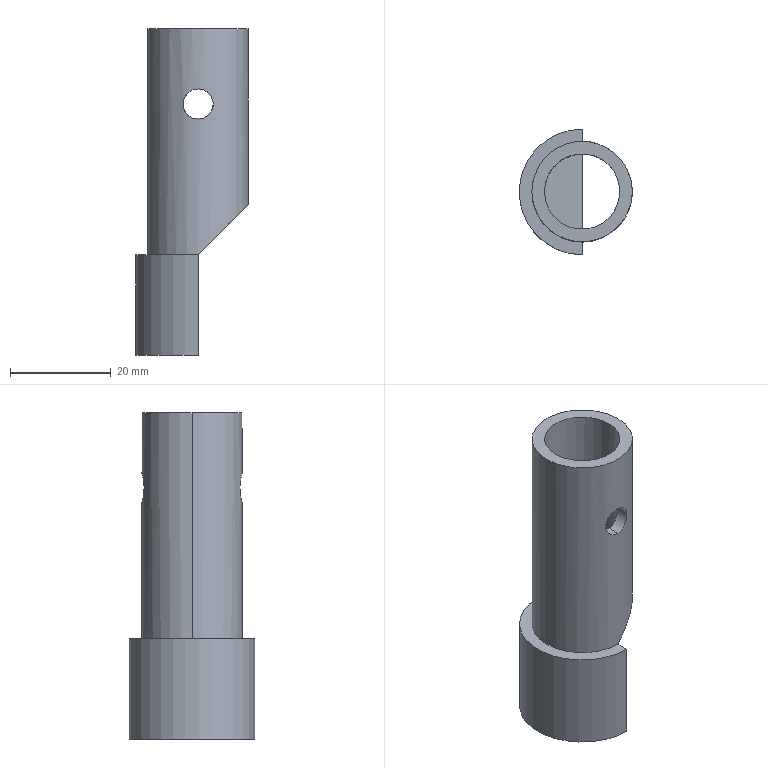Part | SolidWorks | features ICE 3, Extrusion 1, RevCut 1 | 1 solid | 17 faces | box 22.5 x 25 x 65 mm | volume 9681 mm3 | cylinder 9 | plane 6 | sphere 2 | commonest cylinder face diameters 6 x4 15 x2 20 x2 25 x1
STEP:
#1=CARTESIAN_POINT('',(0.,0.,-2.5));
#2=VERTEX_POINT('',#1);
#3=CARTESIAN_POINT('',(0.,0.,-17.5));
#4=VERTEX_POINT('',#3);
#5=CARTESIAN_POINT('',(0.,0.,-10.));
#6=DIRECTION('',(1.,0.,0.));
#7=DIRECTION('',(0.,0.,1.));
#8=AXIS2_PLACEMENT_3D('',#5,#6,#7);
#9=CIRCLE('',#8,7.5);
#10=EDGE_CURVE('',#2,#4,#9,.T.);
#11=ORIENTED_EDGE('',*,*,#10,.T.);
#12=CARTESIAN_POINT('',(0.,0.,-10.));
#13=DIRECTION('',(0.,1.,0.));
#14=DIRECTION('',(0.,0.,1.));
#15=AXIS2_PLACEMENT_3D('',#12,#13,#14);
#16=CIRCLE('',#15,7.5);
#17=EDGE_CURVE('',#4,#2,#16,.T.);
#18=ORIENTED_EDGE('',*,*,#17,.T.);
#19=EDGE_LOOP('',(#11,#18));
#20=FACE_OUTER_BOUND('',#19,.T.);
#21=CARTESIAN_POINT('',(0.,0.,-10.));
#22=DIRECTION('',(0.,-1.,0.));
#23=DIRECTION('',(-1.,0.,0.));
#24=AXIS2_PLACEMENT_3D('',#21,#22,#23);
#25=SPHERICAL_SURFACE('',#24,7.5);
#26=ADVANCED_FACE('',(#20),#25,.F.);
#27=CARTESIAN_POINT('',(0.,-10.,27.));
#28=VERTEX_POINT('',#27);
#29=CARTESIAN_POINT('',(0.,-10.,33.));
#30=VERTEX_POINT('',#29);
#31=CARTESIAN_POINT('',(0.,-10.,27.));
#32=CARTESIAN_POINT('',(-0.1965,-10.,27.));
#33=CARTESIAN_POINT('',(-0.3936,-9.994,27.019));
#34=CARTESIAN_POINT('',(-0.783,-9.971,27.097));
#35=CARTESIAN_POINT('',(-0.9706,-9.954,27.155));
#36=CARTESIAN_POINT('',(-1.332,-9.913,27.305));
#37=CARTESIAN_POINT('',(-1.508,-9.887,27.399));
#38=CARTESIAN_POINT('',(-1.832,-9.832,27.617));
#39=CARTESIAN_POINT('',(-1.983,-9.803,27.74));
#40=CARTESIAN_POINT('',(-2.259,-9.742,28.017));
#41=CARTESIAN_POINT('',(-2.385,-9.712,28.169));
#42=CARTESIAN_POINT('',(-2.601,-9.656,28.493));
#43=CARTESIAN_POINT('',(-2.694,-9.631,28.665));
#44=CARTESIAN_POINT('',(-2.846,-9.587,29.031));
#45=CARTESIAN_POINT('',(-2.903,-9.569,29.218));
#46=CARTESIAN_POINT('',(-2.98,-9.546,29.603));
#47=CARTESIAN_POINT('',(-3.,-9.539,29.802));
#48=CARTESIAN_POINT('',(-3.,-9.539,30.198));
#49=CARTESIAN_POINT('',(-2.981,-9.546,30.393));
#50=CARTESIAN_POINT('',(-2.904,-9.569,30.78));
#51=CARTESIAN_POINT('',(-2.845,-9.587,30.971));
#52=CARTESIAN_POINT('',(-2.62,-9.652,31.513));
#53=CARTESIAN_POINT('',(-2.397,-9.713,31.845));
#54=CARTESIAN_POINT('',(-1.985,-9.802,32.258));
#55=CARTESIAN_POINT('',(-1.832,-9.832,32.384));
#56=CARTESIAN_POINT('',(-1.507,-9.887,32.602));
#57=CARTESIAN_POINT('',(-1.335,-9.912,32.694));
#58=CARTESIAN_POINT('',(-0.973,-9.954,32.845));
#59=CARTESIAN_POINT('',(-0.7815,-9.971,32.903));
#60=CARTESIAN_POINT('',(-0.3956,-9.994,32.98));
#61=CARTESIAN_POINT('',(-0.1994,-10.,33.));
#62=CARTESIAN_POINT('',(0.,-10.,33.));
#63=B_SPLINE_CURVE_WITH_KNOTS('',3,(#31,#32,#33,#34,#35,#36,#37,#38,#39,#40,#41,#42,#43,#44,#45,#46,#47,#48,#49,#50,#51,#52,#53,#54,#55,#56,#57,#58,#59,#60,#61,#62),.UNSPECIFIED.,.F.,.F.,(4,2,2,2,2,2,2,2,2,2,2,2,2,2,2,4),(0.009434,0.01002,0.01061,0.0112,0.01179,0.01238,0.01297,0.01356,0.01415,0.01474,0.01533,0.01651,0.0171,0.01769,0.01828,0.01887),.UNSPECIFIED.);
#64=EDGE_CURVE('',#28,#30,#63,.T.);
#65=ORIENTED_EDGE('',*,*,#64,.F.);
#66=CARTESIAN_POINT('',(0.,-7.5,27.));
#67=VERTEX_POINT('',#66);
#68=CARTESIAN_POINT('',(0.,-10.,27.));
#69=DIRECTION('',(0.,1.,0.));
#70=VECTOR('',#69,1000.);
#71=LINE('',#68,#70);
#72=EDGE_CURVE('',#28,#67,#71,.T.);
#73=ORIENTED_EDGE('',*,*,#72,.T.);
#74=CARTESIAN_POINT('',(0.,-7.5,33.));
#75=VERTEX_POINT('',#74);
#76=CARTESIAN_POINT('',(0.,-7.5,27.));
#77=CARTESIAN_POINT('',(-0.1973,-7.5,27.));
#78=CARTESIAN_POINT('',(-0.3974,-7.492,27.02));
#79=CARTESIAN_POINT('',(-0.7861,-7.461,27.098));
#80=CARTESIAN_POINT('',(-0.9739,-7.439,27.156));
#81=CARTESIAN_POINT('',(-1.337,-7.382,27.307));
#82=CARTESIAN_POINT('',(-1.511,-7.348,27.401));
#83=CARTESIAN_POINT('',(-1.834,-7.274,27.618));
#84=CARTESIAN_POINT('',(-1.985,-7.234,27.742));
#85=CARTESIAN_POINT('',(-2.261,-7.152,28.019));
#86=CARTESIAN_POINT('',(-2.384,-7.112,28.168));
#87=CARTESIAN_POINT('',(-2.6,-7.036,28.49));
#88=CARTESIAN_POINT('',(-2.694,-7.,28.665));
#89=CARTESIAN_POINT('',(-2.845,-6.94,29.027));
#90=CARTESIAN_POINT('',(-2.902,-6.916,29.214));
#91=CARTESIAN_POINT('',(-2.98,-6.883,29.601));
#92=CARTESIAN_POINT('',(-3.,-6.874,29.802));
#93=CARTESIAN_POINT('',(-3.,-6.874,30.197));
#94=CARTESIAN_POINT('',(-2.981,-6.882,30.394));
#95=CARTESIAN_POINT('',(-2.902,-6.916,30.785));
#96=CARTESIAN_POINT('',(-2.844,-6.94,30.974));
#97=CARTESIAN_POINT('',(-2.694,-7.,31.335));
#98=CARTESIAN_POINT('',(-2.6,-7.036,31.509));
#99=CARTESIAN_POINT('',(-2.383,-7.112,31.833));
#100=CARTESIAN_POINT('',(-2.26,-7.153,31.983));
#101=CARTESIAN_POINT('',(-1.985,-7.234,32.258));
#102=CARTESIAN_POINT('',(-1.833,-7.275,32.383));
#103=CARTESIAN_POINT('',(-1.51,-7.348,32.599));
#104=CARTESIAN_POINT('',(-1.339,-7.382,32.692));
#105=CARTESIAN_POINT('',(-0.9736,-7.439,32.845));
#106=CARTESIAN_POINT('',(-0.7847,-7.461,32.902));
#107=CARTESIAN_POINT('',(-0.3992,-7.492,32.98));
#108=CARTESIAN_POINT('',(-0.2004,-7.5,33.));
#109=CARTESIAN_POINT('',(0.,-7.5,33.));
#110=B_SPLINE_CURVE_WITH_KNOTS('',3,(#76,#77,#78,#79,#80,#81,#82,#83,#84,#85,#86,#87,#88,#89,#90,#91,#92,#93,#94,#95,#96,#97,#98,#99,#100,#101,#102,#103,#104,#105,#106,#107,#108,#109),.UNSPECIFIED.,.F.,.F.,(4,2,2,2,2,2,2,2,2,2,2,2,2,2,2,2,4),(0.00948,0.01007,0.01066,0.01126,0.01185,0.01244,0.01303,0.01362,0.01422,0.01481,0.0154,0.01599,0.01658,0.01718,0.01777,0.01836,0.01895),.UNSPECIFIED.);
#111=EDGE_CURVE('',#67,#75,#110,.T.);
#112=ORIENTED_EDGE('',*,*,#111,.T.);
#113=CARTESIAN_POINT('',(0.,-10.,33.));
#114=DIRECTION('',(0.,1.,0.));
#115=VECTOR('',#114,1000.);
#116=LINE('',#113,#115);
#117=EDGE_CURVE('',#30,#75,#116,.T.);
#118=ORIENTED_EDGE('',*,*,#117,.F.);
#119=EDGE_LOOP('',(#65,#73,#112,#118));
#120=FACE_OUTER_BOUND('',#119,.T.);
#121=CARTESIAN_POINT('',(0.,-10.,30.));
#122=DIRECTION('',(0.,1.,0.));
#123=DIRECTION('',(0.,0.,1.));
#124=AXIS2_PLACEMENT_3D('',#121,#122,#123);
#125=CYLINDRICAL_SURFACE('',#124,3.);
#126=ADVANCED_FACE('',(#120),#125,.F.);
#127=CARTESIAN_POINT('',(0.,7.5,33.));
#128=VERTEX_POINT('',#127);
#129=CARTESIAN_POINT('',(0.,7.5,27.));
#130=VERTEX_POINT('',#129);
#131=CARTESIAN_POINT('',(0.,7.5,33.));
#132=CARTESIAN_POINT('',(-0.2005,7.5,33.));
#133=CARTESIAN_POINT('',(-0.3972,7.492,32.98));
#134=CARTESIAN_POINT('',(-0.7836,7.461,32.903));
#135=CARTESIAN_POINT('',(-0.9753,7.439,32.844));
#136=CARTESIAN_POINT('',(-1.338,7.382,32.692));
#137=CARTESIAN_POINT('',(-1.509,7.348,32.6));
#138=CARTESIAN_POINT('',(-1.834,7.274,32.382));
#139=CARTESIAN_POINT('',(-1.986,7.234,32.257));
#140=CARTESIAN_POINT('',(-2.396,7.113,31.846));
#141=CARTESIAN_POINT('',(-2.618,7.03,31.515));
#142=CARTESIAN_POINT('',(-2.844,6.94,30.975));
#143=CARTESIAN_POINT('',(-2.902,6.916,30.784));
#144=CARTESIAN_POINT('',(-2.98,6.883,30.396));
#145=CARTESIAN_POINT('',(-3.,6.874,30.2));
#146=CARTESIAN_POINT('',(-3.,6.874,29.804));
#147=CARTESIAN_POINT('',(-2.98,6.883,29.603));
#148=CARTESIAN_POINT('',(-2.902,6.916,29.216));
#149=CARTESIAN_POINT('',(-2.845,6.94,29.028));
#150=CARTESIAN_POINT('',(-2.692,7.001,28.662));
#151=CARTESIAN_POINT('',(-2.6,7.036,28.491));
#152=CARTESIAN_POINT('',(-2.383,7.112,28.168));
#153=CARTESIAN_POINT('',(-2.258,7.153,28.015));
#154=CARTESIAN_POINT('',(-1.983,7.234,27.741));
#155=CARTESIAN_POINT('',(-1.834,7.274,27.618));
#156=CARTESIAN_POINT('',(-1.51,7.348,27.4));
#157=CARTESIAN_POINT('',(-1.335,7.383,27.306));
#158=CARTESIAN_POINT('',(-0.974,7.439,27.156));
#159=CARTESIAN_POINT('',(-0.7864,7.461,27.098));
#160=CARTESIAN_POINT('',(-0.3955,7.492,27.02));
#161=CARTESIAN_POINT('',(-0.1975,7.5,27.));
#162=CARTESIAN_POINT('',(0.,7.5,27.));
#163=B_SPLINE_CURVE_WITH_KNOTS('',3,(#131,#132,#133,#134,#135,#136,#137,#138,#139,#140,#141,#142,#143,#144,#145,#146,#147,#148,#149,#150,#151,#152,#153,#154,#155,#156,#157,#158,#159,#160,#161,#162),.UNSPECIFIED.,.F.,.F.,(4,2,2,2,2,2,2,2,2,2,2,2,2,2,2,4),(0.,0.0005925,0.001185,0.001777,0.00237,0.003555,0.004147,0.00474,0.005332,0.005925,0.006517,0.00711,0.007702,0.008295,0.008887,0.00948),.UNSPECIFIED.);
#164=EDGE_CURVE('',#128,#130,#163,.T.);
#165=ORIENTED_EDGE('',*,*,#164,.T.);
#166=CARTESIAN_POINT('',(0.,10.,27.));
#167=VERTEX_POINT('',#166);
#168=CARTESIAN_POINT('',(0.,-10.,27.));
#169=DIRECTION('',(0.,1.,0.));
#170=VECTOR('',#169,1000.);
#171=LINE('',#168,#170);
#172=EDGE_CURVE('',#130,#167,#171,.T.);
#173=ORIENTED_EDGE('',*,*,#172,.T.);
#174=CARTESIAN_POINT('',(0.,10.,33.));
#175=VERTEX_POINT('',#174);
#176=CARTESIAN_POINT('',(0.,10.,33.));
#177=CARTESIAN_POINT('',(-0.1995,10.,33.));
#178=CARTESIAN_POINT('',(-0.3954,9.994,32.98));
#179=CARTESIAN_POINT('',(-0.7804,9.971,32.903));
#180=CARTESIAN_POINT('',(-0.9716,9.954,32.845));
#181=CARTESIAN_POINT('',(-1.334,9.912,32.694));
#182=CARTESIAN_POINT('',(-1.506,9.887,32.602));
#183=CARTESIAN_POINT('',(-1.832,9.832,32.384));
#184=CARTESIAN_POINT('',(-1.985,9.802,32.258));
#185=CARTESIAN_POINT('',(-2.397,9.713,31.845));
#186=CARTESIAN_POINT('',(-2.62,9.652,31.513));
#187=CARTESIAN_POINT('',(-2.845,9.587,30.972));
#188=CARTESIAN_POINT('',(-2.903,9.569,30.782));
#189=CARTESIAN_POINT('',(-2.981,9.546,30.394));
#190=CARTESIAN_POINT('',(-3.,9.539,30.198));
#191=CARTESIAN_POINT('',(-3.,9.539,29.804));
#192=CARTESIAN_POINT('',(-2.98,9.546,29.604));
#193=CARTESIAN_POINT('',(-2.903,9.569,29.219));
#194=CARTESIAN_POINT('',(-2.846,9.587,29.031));
#195=CARTESIAN_POINT('',(-2.694,9.63,28.666));
#196=CARTESIAN_POINT('',(-2.601,9.656,28.493));
#197=CARTESIAN_POINT('',(-2.384,9.712,28.169));
#198=CARTESIAN_POINT('',(-2.259,9.743,28.016));
#199=CARTESIAN_POINT('',(-1.982,9.803,27.74));
#200=CARTESIAN_POINT('',(-1.832,9.832,27.616));
#201=CARTESIAN_POINT('',(-1.508,9.887,27.399));
#202=CARTESIAN_POINT('',(-1.332,9.913,27.305));
#203=CARTESIAN_POINT('',(-0.9703,9.954,27.154));
#204=CARTESIAN_POINT('',(-0.7831,9.971,27.097));
#205=CARTESIAN_POINT('',(-0.3956,9.994,27.02));
#206=CARTESIAN_POINT('',(-0.1965,10.,27.));
#207=CARTESIAN_POINT('',(0.,10.,27.));
#208=B_SPLINE_CURVE_WITH_KNOTS('',3,(#176,#177,#178,#179,#180,#181,#182,#183,#184,#185,#186,#187,#188,#189,#190,#191,#192,#193,#194,#195,#196,#197,#198,#199,#200,#201,#202,#203,#204,#205,#206,#207),.UNSPECIFIED.,.F.,.F.,(4,2,2,2,2,2,2,2,2,2,2,2,2,2,2,4),(0.,0.0005896,0.001179,0.001769,0.002359,0.003538,0.004127,0.004717,0.005307,0.005896,0.006486,0.007076,0.007665,0.008255,0.008844,0.009434),.UNSPECIFIED.);
#209=EDGE_CURVE('',#175,#167,#208,.T.);
#210=ORIENTED_EDGE('',*,*,#209,.F.);
#211=CARTESIAN_POINT('',(0.,-10.,33.));
#212=DIRECTION('',(0.,1.,0.));
#213=VECTOR('',#212,1000.);
#214=LINE('',#211,#213);
#215=EDGE_CURVE('',#128,#175,#214,.T.);
#216=ORIENTED_EDGE('',*,*,#215,.F.);
#217=EDGE_LOOP('',(#165,#173,#210,#216));
#218=FACE_OUTER_BOUND('',#217,.T.);
#219=CARTESIAN_POINT('',(0.,-10.,30.));
#220=DIRECTION('',(0.,1.,0.));
#221=DIRECTION('',(0.,0.,1.));
#222=AXIS2_PLACEMENT_3D('',#219,#220,#221);
#223=CYLINDRICAL_SURFACE('',#222,3.);
#224=ADVANCED_FACE('',(#218),#223,.F.);
#225=CARTESIAN_POINT('',(0.,-7.5,33.));
#226=CARTESIAN_POINT('',(0.2005,-7.5,33.));
#227=CARTESIAN_POINT('',(0.3972,-7.492,32.98));
#228=CARTESIAN_POINT('',(0.7836,-7.461,32.903));
#229=CARTESIAN_POINT('',(0.9753,-7.439,32.844));
#230=CARTESIAN_POINT('',(1.338,-7.382,32.692));
#231=CARTESIAN_POINT('',(1.509,-7.348,32.6));
#232=CARTESIAN_POINT('',(1.834,-7.274,32.382));
#233=CARTESIAN_POINT('',(1.986,-7.234,32.257));
#234=CARTESIAN_POINT('',(2.396,-7.113,31.846));
#235=CARTESIAN_POINT('',(2.618,-7.03,31.515));
#236=CARTESIAN_POINT('',(2.844,-6.94,30.975));
#237=CARTESIAN_POINT('',(2.902,-6.916,30.784));
#238=CARTESIAN_POINT('',(2.98,-6.883,30.396));
#239=CARTESIAN_POINT('',(3.,-6.874,30.2));
#240=CARTESIAN_POINT('',(3.,-6.874,29.804));
#241=CARTESIAN_POINT('',(2.98,-6.883,29.603));
#242=CARTESIAN_POINT('',(2.902,-6.916,29.216));
#243=CARTESIAN_POINT('',(2.845,-6.94,29.028));
#244=CARTESIAN_POINT('',(2.692,-7.001,28.662));
#245=CARTESIAN_POINT('',(2.6,-7.036,28.491));
#246=CARTESIAN_POINT('',(2.383,-7.112,28.168));
#247=CARTESIAN_POINT('',(2.258,-7.153,28.015));
#248=CARTESIAN_POINT('',(1.983,-7.234,27.741));
#249=CARTESIAN_POINT('',(1.834,-7.274,27.618));
#250=CARTESIAN_POINT('',(1.51,-7.348,27.4));
#251=CARTESIAN_POINT('',(1.335,-7.383,27.306));
#252=CARTESIAN_POINT('',(0.974,-7.439,27.156));
#253=CARTESIAN_POINT('',(0.7864,-7.461,27.098));
#254=CARTESIAN_POINT('',(0.3955,-7.492,27.02));
#255=CARTESIAN_POINT('',(0.1975,-7.5,27.));
#256=CARTESIAN_POINT('',(0.,-7.5,27.));
#257=B_SPLINE_CURVE_WITH_KNOTS('',3,(#225,#226,#227,#228,#229,#230,#231,#232,#233,#234,#235,#236,#237,#238,#239,#240,#241,#242,#243,#244,#245,#246,#247,#248,#249,#250,#251,#252,#253,#254,#255,#256),.UNSPECIFIED.,.F.,.F.,(4,2,2,2,2,2,2,2,2,2,2,2,2,2,2,4),(0.,0.0005925,0.001185,0.001777,0.00237,0.003555,0.004147,0.00474,0.005332,0.005925,0.006517,0.00711,0.007702,0.008295,0.008887,0.00948),.UNSPECIFIED.);
#258=EDGE_CURVE('',#75,#67,#257,.T.);
#259=ORIENTED_EDGE('',*,*,#258,.F.);
#260=ORIENTED_EDGE('',*,*,#111,.F.);
#261=EDGE_LOOP('',(#259,#260));
#262=FACE_BOUND('',#261,.T.);
#263=CARTESIAN_POINT('',(-7.5,0.,45.));
#264=VERTEX_POINT('',#263);
#265=CARTESIAN_POINT('',(7.5,0.,45.));
#266=VERTEX_POINT('',#265);
#267=CARTESIAN_POINT('',(0.,0.,45.));
#268=DIRECTION('',(0.,0.,1.));
#269=DIRECTION('',(1.,0.,0.));
#270=AXIS2_PLACEMENT_3D('',#267,#268,#269);
#271=CIRCLE('',#270,7.5);
#272=EDGE_CURVE('',#264,#266,#271,.T.);
#273=ORIENTED_EDGE('',*,*,#272,.T.);
#274=CARTESIAN_POINT('',(7.5,0.,7.5));
#275=VERTEX_POINT('',#274);
#276=CARTESIAN_POINT('',(7.5,0.,45.));
#277=DIRECTION('',(0.,0.,-1.));
#278=VECTOR('',#277,1000.);
#279=LINE('',#276,#278);
#280=EDGE_CURVE('',#266,#275,#279,.T.);
#281=ORIENTED_EDGE('',*,*,#280,.T.);
#282=CARTESIAN_POINT('',(0.,-7.5,0.));
#283=VERTEX_POINT('',#282);
#284=CARTESIAN_POINT('',(0.,-7.5,0.));
#285=CARTESIAN_POINT('',(4.393,-7.5,4.393));
#286=CARTESIAN_POINT('',(7.5,-4.393,7.5));
#287=CARTESIAN_POINT('',(7.5,0.,7.5));
#288=(BOUNDED_CURVE()B_SPLINE_CURVE(3,(#284,#285,#286,#287),.UNSPECIFIED.,.F.,.F.)B_SPLINE_CURVE_WITH_KNOTS((4,4),(1.571,3.142),.UNSPECIFIED.)CURVE()GEOMETRIC_REPRESENTATION_ITEM()RATIONAL_B_SPLINE_CURVE((1.,0.8047,0.8047,1.))REPRESENTATION_ITEM(''));
#289=EDGE_CURVE('',#283,#275,#288,.T.);
#290=ORIENTED_EDGE('',*,*,#289,.F.);
#291=CARTESIAN_POINT('',(-7.5,0.,0.));
#292=VERTEX_POINT('',#291);
#293=CARTESIAN_POINT('',(0.,0.,0.));
#294=DIRECTION('',(0.,0.,1.));
#295=DIRECTION('',(1.,0.,0.));
#296=AXIS2_PLACEMENT_3D('',#293,#294,#295);
#297=CIRCLE('',#296,7.5);
#298=EDGE_CURVE('',#292,#283,#297,.T.);
#299=ORIENTED_EDGE('',*,*,#298,.F.);
#300=CARTESIAN_POINT('',(-7.5,0.,45.));
#301=DIRECTION('',(0.,0.,-1.));
#302=VECTOR('',#301,1000.);
#303=LINE('',#300,#302);
#304=EDGE_CURVE('',#264,#292,#303,.T.);
#305=ORIENTED_EDGE('',*,*,#304,.F.);
#306=EDGE_LOOP('',(#273,#281,#290,#299,#305));
#307=FACE_OUTER_BOUND('',#306,.T.);
#308=CARTESIAN_POINT('',(0.,0.,45.));
#309=DIRECTION('',(0.,0.,-1.));
#310=DIRECTION('',(-1.,0.,0.));
#311=AXIS2_PLACEMENT_3D('',#308,#309,#310);
#312=CYLINDRICAL_SURFACE('',#311,7.5);
#313=ADVANCED_FACE('',(#262,#307),#312,.F.);
#314=ORIENTED_EDGE('',*,*,#209,.T.);
#315=CARTESIAN_POINT('',(0.,10.,27.));
#316=CARTESIAN_POINT('',(0.1965,10.,27.));
#317=CARTESIAN_POINT('',(0.3936,9.994,27.019));
#318=CARTESIAN_POINT('',(0.783,9.971,27.097));
#319=CARTESIAN_POINT('',(0.9706,9.954,27.155));
#320=CARTESIAN_POINT('',(1.332,9.913,27.305));
#321=CARTESIAN_POINT('',(1.508,9.887,27.399));
#322=CARTESIAN_POINT('',(1.832,9.832,27.617));
#323=CARTESIAN_POINT('',(1.983,9.803,27.74));
#324=CARTESIAN_POINT('',(2.259,9.742,28.017));
#325=CARTESIAN_POINT('',(2.385,9.712,28.169));
#326=CARTESIAN_POINT('',(2.601,9.656,28.493));
#327=CARTESIAN_POINT('',(2.694,9.631,28.665));
#328=CARTESIAN_POINT('',(2.846,9.587,29.031));
#329=CARTESIAN_POINT('',(2.903,9.569,29.218));
#330=CARTESIAN_POINT('',(2.98,9.546,29.603));
#331=CARTESIAN_POINT('',(3.,9.539,29.802));
#332=CARTESIAN_POINT('',(3.,9.539,30.198));
#333=CARTESIAN_POINT('',(2.981,9.546,30.393));
#334=CARTESIAN_POINT('',(2.904,9.569,30.78));
#335=CARTESIAN_POINT('',(2.845,9.587,30.971));
#336=CARTESIAN_POINT('',(2.62,9.652,31.513));
#337=CARTESIAN_POINT('',(2.397,9.713,31.845));
#338=CARTESIAN_POINT('',(1.985,9.802,32.258));
#339=CARTESIAN_POINT('',(1.832,9.832,32.384));
#340=CARTESIAN_POINT('',(1.507,9.887,32.602));
#341=CARTESIAN_POINT('',(1.335,9.912,32.694));
#342=CARTESIAN_POINT('',(0.973,9.954,32.845));
#343=CARTESIAN_POINT('',(0.7815,9.971,32.903));
#344=CARTESIAN_POINT('',(0.3956,9.994,32.98));
#345=CARTESIAN_POINT('',(0.1994,10.,33.));
#346=CARTESIAN_POINT('',(0.,10.,33.));
#347=B_SPLINE_CURVE_WITH_KNOTS('',3,(#315,#316,#317,#318,#319,#320,#321,#322,#323,#324,#325,#326,#327,#328,#329,#330,#331,#332,#333,#334,#335,#336,#337,#338,#339,#340,#341,#342,#343,#344,#345,#346),.UNSPECIFIED.,.F.,.F.,(4,2,2,2,2,2,2,2,2,2,2,2,2,2,2,4),(0.009434,0.01002,0.01061,0.0112,0.01179,0.01238,0.01297,0.01356,0.01415,0.01474,0.01533,0.01651,0.0171,0.01769,0.01828,0.01887),.UNSPECIFIED.);
#348=EDGE_CURVE('',#167,#175,#347,.T.);
#349=ORIENTED_EDGE('',*,*,#348,.T.);
#350=EDGE_LOOP('',(#314,#349));
#351=FACE_BOUND('',#350,.T.);
#352=CARTESIAN_POINT('',(10.,0.,45.));
#353=VERTEX_POINT('',#352);
#354=CARTESIAN_POINT('',(-10.,0.,45.));
#355=VERTEX_POINT('',#354);
#356=CARTESIAN_POINT('',(0.,0.,45.));
#357=DIRECTION('',(0.,0.,1.));
#358=DIRECTION('',(1.,0.,0.));
#359=AXIS2_PLACEMENT_3D('',#356,#357,#358);
#360=CIRCLE('',#359,10.);
#361=EDGE_CURVE('',#353,#355,#360,.T.);
#362=ORIENTED_EDGE('',*,*,#361,.F.);
#363=CARTESIAN_POINT('',(10.,0.,10.));
#364=VERTEX_POINT('',#363);
#365=CARTESIAN_POINT('',(10.,0.,45.));
#366=DIRECTION('',(0.,0.,-1.));
#367=VECTOR('',#366,1000.);
#368=LINE('',#365,#367);
#369=EDGE_CURVE('',#353,#364,#368,.T.);
#370=ORIENTED_EDGE('',*,*,#369,.T.);
#371=CARTESIAN_POINT('',(0.,10.,0.));
#372=VERTEX_POINT('',#371);
#373=CARTESIAN_POINT('',(10.,0.,10.));
#374=CARTESIAN_POINT('',(10.,5.858,10.));
#375=CARTESIAN_POINT('',(5.858,10.,5.858));
#376=CARTESIAN_POINT('',(0.,10.,0.));
#377=(BOUNDED_CURVE()B_SPLINE_CURVE(3,(#373,#374,#375,#376),.UNSPECIFIED.,.F.,.F.)B_SPLINE_CURVE_WITH_KNOTS((4,4),(3.142,4.712),.UNSPECIFIED.)CURVE()GEOMETRIC_REPRESENTATION_ITEM()RATIONAL_B_SPLINE_CURVE((1.,0.8047,0.8047,1.))REPRESENTATION_ITEM(''));
#378=EDGE_CURVE('',#364,#372,#377,.T.);
#379=ORIENTED_EDGE('',*,*,#378,.T.);
#380=CARTESIAN_POINT('',(-10.,0.,0.));
#381=VERTEX_POINT('',#380);
#382=CARTESIAN_POINT('',(0.,0.,0.));
#383=DIRECTION('',(0.,0.,-1.));
#384=DIRECTION('',(-1.,0.,0.));
#385=AXIS2_PLACEMENT_3D('',#382,#383,#384);
#386=CIRCLE('',#385,10.);
#387=EDGE_CURVE('',#381,#372,#386,.T.);
#388=ORIENTED_EDGE('',*,*,#387,.F.);
#389=CARTESIAN_POINT('',(-10.,0.,45.));
#390=DIRECTION('',(0.,0.,-1.));
#391=VECTOR('',#390,1000.);
#392=LINE('',#389,#391);
#393=EDGE_CURVE('',#355,#381,#392,.T.);
#394=ORIENTED_EDGE('',*,*,#393,.F.);
#395=EDGE_LOOP('',(#362,#370,#379,#388,#394));
#396=FACE_OUTER_BOUND('',#395,.T.);
#397=CARTESIAN_POINT('',(0.,0.,45.));
#398=DIRECTION('',(0.,0.,-1.));
#399=DIRECTION('',(-1.,0.,0.));
#400=AXIS2_PLACEMENT_3D('',#397,#398,#399);
#401=CYLINDRICAL_SURFACE('',#400,10.);
#402=ADVANCED_FACE('',(#351,#396),#401,.T.);
#403=CARTESIAN_POINT('',(0.,0.,45.));
#404=DIRECTION('',(0.,0.,1.));
#405=DIRECTION('',(1.,0.,0.));
#406=AXIS2_PLACEMENT_3D('',#403,#404,#405);
#407=CIRCLE('',#406,10.);
#408=EDGE_CURVE('',#355,#353,#407,.T.);
#409=ORIENTED_EDGE('',*,*,#408,.T.);
#410=ORIENTED_EDGE('',*,*,#361,.T.);
#411=EDGE_LOOP('',(#409,#410));
#412=FACE_OUTER_BOUND('',#411,.T.);
#413=ORIENTED_EDGE('',*,*,#272,.F.);
#414=CARTESIAN_POINT('',(0.,0.,45.));
#415=DIRECTION('',(0.,0.,1.));
#416=DIRECTION('',(1.,0.,0.));
#417=AXIS2_PLACEMENT_3D('',#414,#415,#416);
#418=CIRCLE('',#417,7.5);
#419=EDGE_CURVE('',#266,#264,#418,.T.);
#420=ORIENTED_EDGE('',*,*,#419,.F.);
#421=EDGE_LOOP('',(#413,#420));
#422=FACE_BOUND('',#421,.T.);
#423=CARTESIAN_POINT('',(0.,0.,45.));
#424=DIRECTION('',(0.,0.,1.));
#425=DIRECTION('',(1.,0.,0.));
#426=AXIS2_PLACEMENT_3D('',#423,#424,#425);
#427=PLANE('',#426);
#428=ADVANCED_FACE('',(#412,#422),#427,.T.);
#429=ORIENTED_EDGE('',*,*,#369,.F.);
#430=ORIENTED_EDGE('',*,*,#408,.F.);
#431=ORIENTED_EDGE('',*,*,#393,.T.);
#432=CARTESIAN_POINT('',(0.,-10.,0.));
#433=VERTEX_POINT('',#432);
#434=CARTESIAN_POINT('',(0.,0.,0.));
#435=DIRECTION('',(0.,0.,-1.));
#436=DIRECTION('',(-1.,0.,0.));
#437=AXIS2_PLACEMENT_3D('',#434,#435,#436);
#438=CIRCLE('',#437,10.);
#439=EDGE_CURVE('',#433,#381,#438,.T.);
#440=ORIENTED_EDGE('',*,*,#439,.F.);
#441=CARTESIAN_POINT('',(0.,-10.,0.));
#442=CARTESIAN_POINT('',(5.858,-10.,5.858));
#443=CARTESIAN_POINT('',(10.,-5.858,10.));
#444=CARTESIAN_POINT('',(10.,0.,10.));
#445=(BOUNDED_CURVE()B_SPLINE_CURVE(3,(#441,#442,#443,#444),.UNSPECIFIED.,.F.,.F.)B_SPLINE_CURVE_WITH_KNOTS((4,4),(1.571,3.142),.UNSPECIFIED.)CURVE()GEOMETRIC_REPRESENTATION_ITEM()RATIONAL_B_SPLINE_CURVE((1.,0.8047,0.8047,1.))REPRESENTATION_ITEM(''));
#446=EDGE_CURVE('',#433,#364,#445,.T.);
#447=ORIENTED_EDGE('',*,*,#446,.T.);
#448=EDGE_LOOP('',(#429,#430,#431,#440,#447));
#449=FACE_OUTER_BOUND('',#448,.T.);
#450=CARTESIAN_POINT('',(0.,-10.,33.));
#451=CARTESIAN_POINT('',(0.1995,-10.,33.));
#452=CARTESIAN_POINT('',(0.3954,-9.994,32.98));
#453=CARTESIAN_POINT('',(0.7804,-9.971,32.903));
#454=CARTESIAN_POINT('',(0.9716,-9.954,32.845));
#455=CARTESIAN_POINT('',(1.334,-9.912,32.694));
#456=CARTESIAN_POINT('',(1.506,-9.887,32.602));
#457=CARTESIAN_POINT('',(1.832,-9.832,32.384));
#458=CARTESIAN_POINT('',(1.985,-9.802,32.258));
#459=CARTESIAN_POINT('',(2.397,-9.713,31.845));
#460=CARTESIAN_POINT('',(2.62,-9.652,31.513));
#461=CARTESIAN_POINT('',(2.845,-9.587,30.972));
#462=CARTESIAN_POINT('',(2.903,-9.569,30.782));
#463=CARTESIAN_POINT('',(2.981,-9.546,30.394));
#464=CARTESIAN_POINT('',(3.,-9.539,30.198));
#465=CARTESIAN_POINT('',(3.,-9.539,29.804));
#466=CARTESIAN_POINT('',(2.98,-9.546,29.604));
#467=CARTESIAN_POINT('',(2.903,-9.569,29.219));
#468=CARTESIAN_POINT('',(2.846,-9.587,29.031));
#469=CARTESIAN_POINT('',(2.694,-9.63,28.666));
#470=CARTESIAN_POINT('',(2.601,-9.656,28.493));
#471=CARTESIAN_POINT('',(2.384,-9.712,28.169));
#472=CARTESIAN_POINT('',(2.259,-9.743,28.016));
#473=CARTESIAN_POINT('',(1.982,-9.803,27.74));
#474=CARTESIAN_POINT('',(1.832,-9.832,27.616));
#475=CARTESIAN_POINT('',(1.508,-9.887,27.399));
#476=CARTESIAN_POINT('',(1.332,-9.913,27.305));
#477=CARTESIAN_POINT('',(0.9703,-9.954,27.154));
#478=CARTESIAN_POINT('',(0.7831,-9.971,27.097));
#479=CARTESIAN_POINT('',(0.3956,-9.994,27.02));
#480=CARTESIAN_POINT('',(0.1965,-10.,27.));
#481=CARTESIAN_POINT('',(0.,-10.,27.));
#482=B_SPLINE_CURVE_WITH_KNOTS('',3,(#450,#451,#452,#453,#454,#455,#456,#457,#458,#459,#460,#461,#462,#463,#464,#465,#466,#467,#468,#469,#470,#471,#472,#473,#474,#475,#476,#477,#478,#479,#480,#481),.UNSPECIFIED.,.F.,.F.,(4,2,2,2,2,2,2,2,2,2,2,2,2,2,2,4),(0.,0.0005896,0.001179,0.001769,0.002359,0.003538,0.004127,0.004717,0.005307,0.005896,0.006486,0.007076,0.007665,0.008255,0.008844,0.009434),.UNSPECIFIED.);
#483=EDGE_CURVE('',#30,#28,#482,.T.);
#484=ORIENTED_EDGE('',*,*,#483,.T.);
#485=ORIENTED_EDGE('',*,*,#64,.T.);
#486=EDGE_LOOP('',(#484,#485));
#487=FACE_BOUND('',#486,.T.);
#488=CARTESIAN_POINT('',(0.,0.,45.));
#489=DIRECTION('',(0.,0.,-1.));
#490=DIRECTION('',(-1.,0.,0.));
#491=AXIS2_PLACEMENT_3D('',#488,#489,#490);
#492=CYLINDRICAL_SURFACE('',#491,10.);
#493=ADVANCED_FACE('',(#449,#487),#492,.T.);
#494=ORIENTED_EDGE('',*,*,#280,.F.);
#495=ORIENTED_EDGE('',*,*,#419,.T.);
#496=ORIENTED_EDGE('',*,*,#304,.T.);
#497=CARTESIAN_POINT('',(0.,7.5,0.));
#498=VERTEX_POINT('',#497);
#499=CARTESIAN_POINT('',(0.,0.,0.));
#500=DIRECTION('',(0.,0.,1.));
#501=DIRECTION('',(1.,0.,0.));
#502=AXIS2_PLACEMENT_3D('',#499,#500,#501);
#503=CIRCLE('',#502,7.5);
#504=EDGE_CURVE('',#498,#292,#503,.T.);
#505=ORIENTED_EDGE('',*,*,#504,.F.);
#506=CARTESIAN_POINT('',(7.5,0.,7.5));
#507=CARTESIAN_POINT('',(7.5,4.393,7.5));
#508=CARTESIAN_POINT('',(4.393,7.5,4.393));
#509=CARTESIAN_POINT('',(0.,7.5,0.));
#510=(BOUNDED_CURVE()B_SPLINE_CURVE(3,(#506,#507,#508,#509),.UNSPECIFIED.,.F.,.F.)B_SPLINE_CURVE_WITH_KNOTS((4,4),(3.142,4.712),.UNSPECIFIED.)CURVE()GEOMETRIC_REPRESENTATION_ITEM()RATIONAL_B_SPLINE_CURVE((1.,0.8047,0.8047,1.))REPRESENTATION_ITEM(''));
#511=EDGE_CURVE('',#275,#498,#510,.T.);
#512=ORIENTED_EDGE('',*,*,#511,.F.);
#513=EDGE_LOOP('',(#494,#495,#496,#505,#512));
#514=FACE_OUTER_BOUND('',#513,.T.);
#515=ORIENTED_EDGE('',*,*,#164,.F.);
#516=CARTESIAN_POINT('',(0.,7.5,27.));
#517=CARTESIAN_POINT('',(0.1973,7.5,27.));
#518=CARTESIAN_POINT('',(0.3974,7.492,27.02));
#519=CARTESIAN_POINT('',(0.7861,7.461,27.098));
#520=CARTESIAN_POINT('',(0.9739,7.439,27.156));
#521=CARTESIAN_POINT('',(1.337,7.382,27.307));
#522=CARTESIAN_POINT('',(1.511,7.348,27.401));
#523=CARTESIAN_POINT('',(1.834,7.274,27.618));
#524=CARTESIAN_POINT('',(1.985,7.234,27.742));
#525=CARTESIAN_POINT('',(2.261,7.152,28.019));
#526=CARTESIAN_POINT('',(2.384,7.112,28.168));
#527=CARTESIAN_POINT('',(2.6,7.036,28.49));
#528=CARTESIAN_POINT('',(2.694,7.,28.665));
#529=CARTESIAN_POINT('',(2.845,6.94,29.027));
#530=CARTESIAN_POINT('',(2.902,6.916,29.214));
#531=CARTESIAN_POINT('',(2.98,6.883,29.601));
#532=CARTESIAN_POINT('',(3.,6.874,29.802));
#533=CARTESIAN_POINT('',(3.,6.874,30.197));
#534=CARTESIAN_POINT('',(2.981,6.882,30.394));
#535=CARTESIAN_POINT('',(2.902,6.916,30.785));
#536=CARTESIAN_POINT('',(2.844,6.94,30.974));
#537=CARTESIAN_POINT('',(2.694,7.,31.335));
#538=CARTESIAN_POINT('',(2.6,7.036,31.509));
#539=CARTESIAN_POINT('',(2.383,7.112,31.833));
#540=CARTESIAN_POINT('',(2.26,7.153,31.983));
#541=CARTESIAN_POINT('',(1.985,7.234,32.258));
#542=CARTESIAN_POINT('',(1.833,7.275,32.383));
#543=CARTESIAN_POINT('',(1.51,7.348,32.599));
#544=CARTESIAN_POINT('',(1.339,7.382,32.692));
#545=CARTESIAN_POINT('',(0.9736,7.439,32.845));
#546=CARTESIAN_POINT('',(0.7847,7.461,32.902));
#547=CARTESIAN_POINT('',(0.3992,7.492,32.98));
#548=CARTESIAN_POINT('',(0.2004,7.5,33.));
#549=CARTESIAN_POINT('',(0.,7.5,33.));
#550=B_SPLINE_CURVE_WITH_KNOTS('',3,(#516,#517,#518,#519,#520,#521,#522,#523,#524,#525,#526,#527,#528,#529,#530,#531,#532,#533,#534,#535,#536,#537,#538,#539,#540,#541,#542,#543,#544,#545,#546,#547,#548,#549),.UNSPECIFIED.,.F.,.F.,(4,2,2,2,2,2,2,2,2,2,2,2,2,2,2,2,4),(0.00948,0.01007,0.01066,0.01126,0.01185,0.01244,0.01303,0.01362,0.01422,0.01481,0.0154,0.01599,0.01658,0.01718,0.01777,0.01836,0.01895),.UNSPECIFIED.);
#551=EDGE_CURVE('',#130,#128,#550,.T.);
#552=ORIENTED_EDGE('',*,*,#551,.F.);
#553=EDGE_LOOP('',(#515,#552));
#554=FACE_BOUND('',#553,.T.);
#555=CARTESIAN_POINT('',(0.,0.,45.));
#556=DIRECTION('',(0.,0.,-1.));
#557=DIRECTION('',(-1.,0.,0.));
#558=AXIS2_PLACEMENT_3D('',#555,#556,#557);
#559=CYLINDRICAL_SURFACE('',#558,7.5);
#560=ADVANCED_FACE('',(#514,#554),#559,.F.);
#561=ORIENTED_EDGE('',*,*,#172,.F.);
#562=ORIENTED_EDGE('',*,*,#551,.T.);
#563=ORIENTED_EDGE('',*,*,#215,.T.);
#564=ORIENTED_EDGE('',*,*,#348,.F.);
#565=EDGE_LOOP('',(#561,#562,#563,#564));
#566=FACE_OUTER_BOUND('',#565,.T.);
#567=CARTESIAN_POINT('',(0.,-10.,30.));
#568=DIRECTION('',(0.,1.,0.));
#569=DIRECTION('',(0.,0.,1.));
#570=AXIS2_PLACEMENT_3D('',#567,#568,#569);
#571=CYLINDRICAL_SURFACE('',#570,3.);
#572=ADVANCED_FACE('',(#566),#571,.F.);
#573=ORIENTED_EDGE('',*,*,#72,.F.);
#574=ORIENTED_EDGE('',*,*,#483,.F.);
#575=ORIENTED_EDGE('',*,*,#117,.T.);
#576=ORIENTED_EDGE('',*,*,#258,.T.);
#577=EDGE_LOOP('',(#573,#574,#575,#576));
#578=FACE_OUTER_BOUND('',#577,.T.);
#579=CARTESIAN_POINT('',(0.,-10.,30.));
#580=DIRECTION('',(0.,1.,0.));
#581=DIRECTION('',(0.,0.,1.));
#582=AXIS2_PLACEMENT_3D('',#579,#580,#581);
#583=CYLINDRICAL_SURFACE('',#582,3.);
#584=ADVANCED_FACE('',(#578),#583,.F.);
#585=ORIENTED_EDGE('',*,*,#504,.T.);
#586=ORIENTED_EDGE('',*,*,#298,.T.);
#587=CARTESIAN_POINT('',(0.,-12.5,0.));
#588=DIRECTION('',(0.,1.,0.));
#589=VECTOR('',#588,1000.);
#590=LINE('',#587,#589);
#591=EDGE_CURVE('',#283,#498,#590,.T.);
#592=ORIENTED_EDGE('',*,*,#591,.T.);
#593=EDGE_LOOP('',(#585,#586,#592));
#594=FACE_OUTER_BOUND('',#593,.T.);
#595=CARTESIAN_POINT('',(0.,0.,0.));
#596=DIRECTION('',(0.,0.,-1.));
#597=DIRECTION('',(-1.,0.,0.));
#598=AXIS2_PLACEMENT_3D('',#595,#596,#597);
#599=PLANE('',#598);
#600=ADVANCED_FACE('',(#594),#599,.F.);
#601=CARTESIAN_POINT('',(0.,-12.5,-20.));
#602=VERTEX_POINT('',#601);
#603=CARTESIAN_POINT('',(0.,12.5,-20.));
#604=VERTEX_POINT('',#603);
#605=CARTESIAN_POINT('',(0.,0.,-20.));
#606=DIRECTION('',(0.,0.,-1.));
#607=DIRECTION('',(-1.,0.,0.));
#608=AXIS2_PLACEMENT_3D('',#605,#606,#607);
#609=CIRCLE('',#608,12.5);
#610=EDGE_CURVE('',#602,#604,#609,.T.);
#611=ORIENTED_EDGE('',*,*,#610,.F.);
#612=CARTESIAN_POINT('',(0.,-12.5,0.));
#613=VERTEX_POINT('',#612);
#614=CARTESIAN_POINT('',(0.,-12.5,-20.));
#615=DIRECTION('',(0.,0.,1.));
#616=VECTOR('',#615,1000.);
#617=LINE('',#614,#616);
#618=EDGE_CURVE('',#602,#613,#617,.T.);
#619=ORIENTED_EDGE('',*,*,#618,.T.);
#620=CARTESIAN_POINT('',(0.,12.5,0.));
#621=VERTEX_POINT('',#620);
#622=CARTESIAN_POINT('',(0.,0.,0.));
#623=DIRECTION('',(0.,0.,-1.));
#624=DIRECTION('',(-1.,0.,0.));
#625=AXIS2_PLACEMENT_3D('',#622,#623,#624);
#626=CIRCLE('',#625,12.5);
#627=EDGE_CURVE('',#613,#621,#626,.T.);
#628=ORIENTED_EDGE('',*,*,#627,.T.);
#629=CARTESIAN_POINT('',(0.,12.5,-20.));
#630=DIRECTION('',(0.,0.,1.));
#631=VECTOR('',#630,1000.);
#632=LINE('',#629,#631);
#633=EDGE_CURVE('',#604,#621,#632,.T.);
#634=ORIENTED_EDGE('',*,*,#633,.F.);
#635=EDGE_LOOP('',(#611,#619,#628,#634));
#636=FACE_OUTER_BOUND('',#635,.T.);
#637=CARTESIAN_POINT('',(0.,0.,-20.));
#638=DIRECTION('',(0.,0.,1.));
#639=DIRECTION('',(1.,0.,0.));
#640=AXIS2_PLACEMENT_3D('',#637,#638,#639);
#641=CYLINDRICAL_SURFACE('',#640,12.5);
#642=ADVANCED_FACE('',(#636),#641,.T.);
#643=CARTESIAN_POINT('',(0.,-12.5,-20.));
#644=DIRECTION('',(0.,1.,0.));
#645=VECTOR('',#644,1000.);
#646=LINE('',#643,#645);
#647=EDGE_CURVE('',#602,#604,#646,.T.);
#648=ORIENTED_EDGE('',*,*,#647,.F.);
#649=ORIENTED_EDGE('',*,*,#610,.T.);
#650=EDGE_LOOP('',(#648,#649));
#651=FACE_OUTER_BOUND('',#650,.T.);
#652=CARTESIAN_POINT('',(0.,0.,-20.));
#653=DIRECTION('',(0.,0.,-1.));
#654=DIRECTION('',(-1.,0.,0.));
#655=AXIS2_PLACEMENT_3D('',#652,#653,#654);
#656=PLANE('',#655);
#657=ADVANCED_FACE('',(#651),#656,.T.);
#658=ORIENTED_EDGE('',*,*,#627,.F.);
#659=CARTESIAN_POINT('',(0.,-12.5,0.));
#660=DIRECTION('',(0.,1.,0.));
#661=VECTOR('',#660,1000.);
#662=LINE('',#659,#661);
#663=EDGE_CURVE('',#613,#433,#662,.T.);
#664=ORIENTED_EDGE('',*,*,#663,.T.);
#665=ORIENTED_EDGE('',*,*,#439,.T.);
#666=ORIENTED_EDGE('',*,*,#387,.T.);
#667=CARTESIAN_POINT('',(0.,0.,0.));
#668=DIRECTION('',(0.,1.,0.));
#669=VECTOR('',#668,1000.);
#670=LINE('',#667,#669);
#671=EDGE_CURVE('',#372,#621,#670,.T.);
#672=ORIENTED_EDGE('',*,*,#671,.T.);
#673=EDGE_LOOP('',(#658,#664,#665,#666,#672));
#674=FACE_OUTER_BOUND('',#673,.T.);
#675=CARTESIAN_POINT('',(0.,0.,0.));
#676=DIRECTION('',(0.,0.,-1.));
#677=DIRECTION('',(-1.,0.,0.));
#678=AXIS2_PLACEMENT_3D('',#675,#676,#677);
#679=PLANE('',#678);
#680=ADVANCED_FACE('',(#674),#679,.F.);
#681=CARTESIAN_POINT('',(0.,-12.5,0.));
#682=DIRECTION('',(0.,1.,0.));
#683=VECTOR('',#682,1000.);
#684=LINE('',#681,#683);
#685=EDGE_CURVE('',#433,#283,#684,.T.);
#686=ORIENTED_EDGE('',*,*,#685,.T.);
#687=ORIENTED_EDGE('',*,*,#289,.T.);
#688=ORIENTED_EDGE('',*,*,#511,.T.);
#689=CARTESIAN_POINT('',(0.,-12.5,0.));
#690=DIRECTION('',(0.,1.,0.));
#691=VECTOR('',#690,1000.);
#692=LINE('',#689,#691);
#693=EDGE_CURVE('',#498,#372,#692,.T.);
#694=ORIENTED_EDGE('',*,*,#693,.T.);
#695=ORIENTED_EDGE('',*,*,#378,.F.);
#696=ORIENTED_EDGE('',*,*,#446,.F.);
#697=EDGE_LOOP('',(#686,#687,#688,#694,#695,#696));
#698=FACE_OUTER_BOUND('',#697,.T.);
#699=CARTESIAN_POINT('',(0.,-12.5,0.));
#700=DIRECTION('',(-0.7071,0.,0.7071));
#701=DIRECTION('',(0.7071,0.,0.7071));
#702=AXIS2_PLACEMENT_3D('',#699,#700,#701);
#703=PLANE('',#702);
#704=ADVANCED_FACE('',(#698),#703,.F.);
#705=ORIENTED_EDGE('',*,*,#10,.F.);
#706=CARTESIAN_POINT('',(0.,0.,-10.));
#707=DIRECTION('',(1.,0.,0.));
#708=DIRECTION('',(0.,0.,1.));
#709=AXIS2_PLACEMENT_3D('',#706,#707,#708);
#710=CIRCLE('',#709,7.5);
#711=EDGE_CURVE('',#4,#2,#710,.T.);
#712=ORIENTED_EDGE('',*,*,#711,.F.);
#713=EDGE_LOOP('',(#705,#712));
#714=FACE_BOUND('',#713,.T.);
#715=ORIENTED_EDGE('',*,*,#663,.F.);
#716=ORIENTED_EDGE('',*,*,#618,.F.);
#717=ORIENTED_EDGE('',*,*,#647,.T.);
#718=ORIENTED_EDGE('',*,*,#633,.T.);
#719=ORIENTED_EDGE('',*,*,#671,.F.);
#720=ORIENTED_EDGE('',*,*,#693,.F.);
#721=ORIENTED_EDGE('',*,*,#591,.F.);
#722=ORIENTED_EDGE('',*,*,#685,.F.);
#723=EDGE_LOOP('',(#715,#716,#717,#718,#719,#720,#721,#722));
#724=FACE_OUTER_BOUND('',#723,.T.);
#725=CARTESIAN_POINT('',(0.,-12.5,-20.));
#726=DIRECTION('',(-1.,0.,0.));
#727=DIRECTION('',(0.,0.,1.));
#728=AXIS2_PLACEMENT_3D('',#725,#726,#727);
#729=PLANE('',#728);
#730=ADVANCED_FACE('',(#714,#724),#729,.F.);
#731=ORIENTED_EDGE('',*,*,#17,.F.);
#732=ORIENTED_EDGE('',*,*,#711,.T.);
#733=EDGE_LOOP('',(#731,#732));
#734=FACE_OUTER_BOUND('',#733,.T.);
#735=CARTESIAN_POINT('',(0.,0.,-10.));
#736=DIRECTION('',(0.,-1.,0.));
#737=DIRECTION('',(-1.,0.,0.));
#738=AXIS2_PLACEMENT_3D('',#735,#736,#737);
#739=SPHERICAL_SURFACE('',#738,7.5);
#740=ADVANCED_FACE('',(#734),#739,.F.);
#741=CLOSED_SHELL('',(#26,#126,#224,#313,#402,#428,#493,#560,#572,#584,#600,#642,#657,#680,#704,#730,#740));
#742=MANIFOLD_SOLID_BREP('',#741);
#743=CARTESIAN_POINT('',(0.,0.,0.));
#744=DIRECTION('',(0.,0.,1.));
#745=DIRECTION('',(1.,0.,0.));
#746=AXIS2_PLACEMENT_3D('',#743,#744,#745);
#747=(LENGTH_UNIT()NAMED_UNIT(*)SI_UNIT(.MILLI.,.METRE.));
#748=UNCERTAINTY_MEASURE_WITH_UNIT(LENGTH_MEASURE(0.00001),#747,'','');
#749=(NAMED_UNIT(*)PLANE_ANGLE_UNIT()SI_UNIT($,.RADIAN.));
#750=(NAMED_UNIT(*)SI_UNIT($,.STERADIAN.)SOLID_ANGLE_UNIT());
#751=(GEOMETRIC_REPRESENTATION_CONTEXT(3)GLOBAL_UNCERTAINTY_ASSIGNED_CONTEXT((#748))GLOBAL_UNIT_ASSIGNED_CONTEXT((#747,#749,#750))REPRESENTATION_CONTEXT('',''));
#752=ADVANCED_BREP_SHAPE_REPRESENTATION('',(#742,#746),#751);